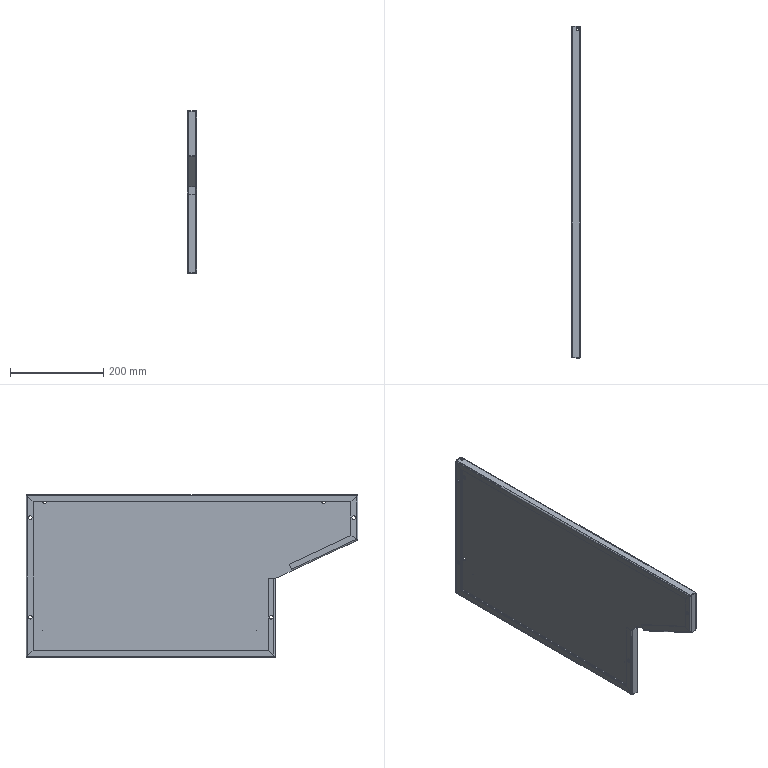Part | NX | features solid 2 | 1 solid | 191 faces | box 20 x 713.5 x 350 mm | volume 406502 mm3 | plane 96 | cylinder 56 | spline 39 | commonest cylinder face diameters 6 x16 8 x16 3 x12 1 x4 7 x4 9.2 x4